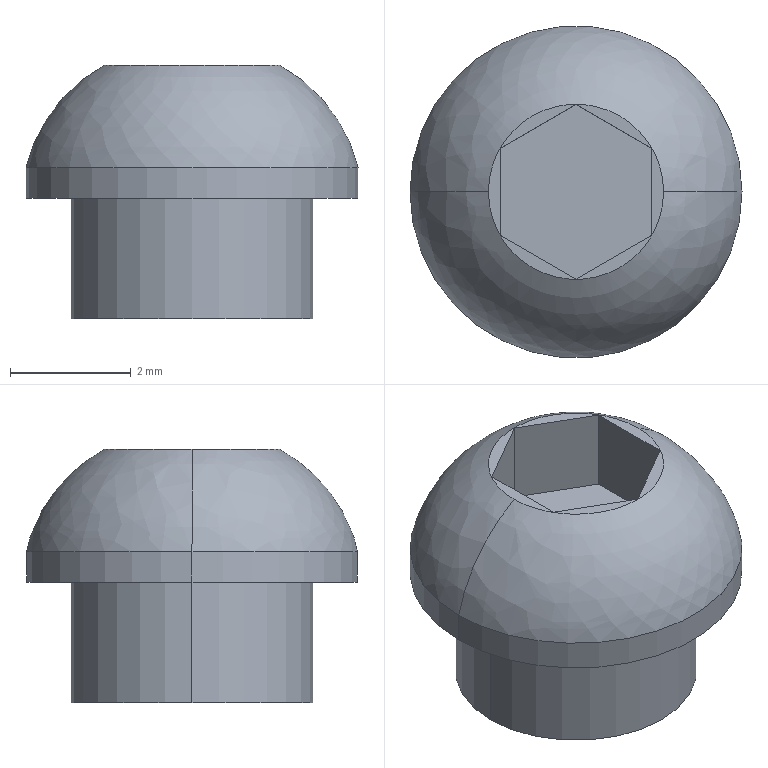Part | STEP file | 1 solid | 16 faces | box 5.5 x 5.5 x 4.2 mm | volume 58.227 mm3 | plane 10 | cylinder 4 | spline 2 | commonest cylinder face diameters 4 x2 5.5 x2
STEP:
#1=CARTESIAN_POINT('',(0.,0.,0.));
#2=DIRECTION('',(0.,0.,1.));
#3=DIRECTION('',(1.,0.,0.));
#4=AXIS2_PLACEMENT_3D('',#1,#2,#3);
#5=CARTESIAN_POINT('',(2.735,0.,5.794));
#6=VERTEX_POINT('',#5);
#7=CARTESIAN_POINT('',(-0.1645,0.,5.794));
#8=VERTEX_POINT('',#7);
#9=CARTESIAN_POINT('',(1.285,0.,5.794));
#10=DIRECTION('',(0.,0.,-1.));
#11=DIRECTION('',(1.,0.,0.));
#12=AXIS2_PLACEMENT_3D('',#9,#10,#11);
#13=CIRCLE('',#12,1.45);
#14=CARTESIAN_POINT('',(-0.1645,0.,5.794));
#15=CARTESIAN_POINT('',(-0.1645,-2.9,5.794));
#16=CARTESIAN_POINT('',(2.735,-2.9,5.794));
#17=CARTESIAN_POINT('',(2.735,0.,5.794));
#18=CARTESIAN_POINT('',(-0.8301,0.,5.432));
#19=CARTESIAN_POINT('',(-0.8301,-4.231,5.432));
#20=CARTESIAN_POINT('',(3.401,-4.231,5.432));
#21=CARTESIAN_POINT('',(3.401,0.,5.432));
#22=CARTESIAN_POINT('',(-1.29,0.,4.831));
#23=CARTESIAN_POINT('',(-1.29,-5.151,4.831));
#24=CARTESIAN_POINT('',(3.861,-5.151,4.831));
#25=CARTESIAN_POINT('',(3.861,0.,4.831));
#26=CARTESIAN_POINT('',(-1.465,0.,4.094));
#27=CARTESIAN_POINT('',(-1.465,-5.5,4.094));
#28=CARTESIAN_POINT('',(4.035,-5.5,4.094));
#29=CARTESIAN_POINT('',(4.035,0.,4.094));
#30=(BOUNDED_SURFACE()B_SPLINE_SURFACE(3,3,((#14,#15,#16,#17),(#18,#19,#20,#21),(#22,#23,#24,#25),(#26,#27,#28,#29)),.UNSPECIFIED.,.F.,.F.,.F.)B_SPLINE_SURFACE_WITH_KNOTS((4,4),(4,4),(0.,1.),(0.,1.),.PIECEWISE_BEZIER_KNOTS.)GEOMETRIC_REPRESENTATION_ITEM()RATIONAL_B_SPLINE_SURFACE(((1.,0.3333,0.3333,1.),(0.9419,0.314,0.314,0.9419),(0.9419,0.314,0.314,0.9419),(1.,0.3333,0.3333,1.)))REPRESENTATION_ITEM('')SURFACE());
#31=CARTESIAN_POINT('',(0.,1.));
#32=CARTESIAN_POINT('',(0.,0.9763));
#33=CARTESIAN_POINT('',(0.,0.9319));
#34=CARTESIAN_POINT('',(0.,0.8733));
#35=CARTESIAN_POINT('',(0.,0.8206));
#36=CARTESIAN_POINT('',(0.,0.7724));
#37=CARTESIAN_POINT('',(0.,0.7279));
#38=CARTESIAN_POINT('',(0.,0.6861));
#39=CARTESIAN_POINT('',(0.,0.6465));
#40=CARTESIAN_POINT('',(0.,0.6086));
#41=CARTESIAN_POINT('',(0.,0.5718));
#42=CARTESIAN_POINT('',(0.,0.5357));
#43=CARTESIAN_POINT('',(0.,0.5));
#44=CARTESIAN_POINT('',(0.,0.4643));
#45=CARTESIAN_POINT('',(0.,0.4282));
#46=CARTESIAN_POINT('',(0.,0.3914));
#47=CARTESIAN_POINT('',(0.,0.3535));
#48=CARTESIAN_POINT('',(0.,0.3139));
#49=CARTESIAN_POINT('',(0.,0.2721));
#50=CARTESIAN_POINT('',(0.,0.2276));
#51=CARTESIAN_POINT('',(0.,0.1794));
#52=CARTESIAN_POINT('',(0.,0.1267));
#53=CARTESIAN_POINT('',(0.,0.06805));
#54=CARTESIAN_POINT('',(0.,0.02375));
#55=CARTESIAN_POINT('',(0.,0.));
#56=B_SPLINE_CURVE_WITH_KNOTS('',3,(#31,#32,#33,#34,#35,#36,#37,#38,#39,#40,#41,#42,#43,#44,#45,#46,#47,#48,#49,#50,#51,#52,#53,#54,#55),.UNSPECIFIED.,.F.,.F.,(4,1,1,1,1,1,1,1,1,1,1,1,1,1,1,1,1,1,1,1,1,1,4),(0.,0.1428,0.2856,0.4284,0.5712,0.714,0.8568,0.9996,1.142,1.285,1.428,1.571,1.714,1.856,1.999,2.142,2.285,2.428,2.57,2.713,2.856,2.999,3.142),.QUASI_UNIFORM_KNOTS.);
#57=(GEOMETRIC_REPRESENTATION_CONTEXT(2)PARAMETRIC_REPRESENTATION_CONTEXT()REPRESENTATION_CONTEXT('',''));
#58=DEFINITIONAL_REPRESENTATION('',(#56),#57);
#59=PCURVE('',#30,#58);
#60=CARTESIAN_POINT('',(1.285,0.,5.794));
#61=DIRECTION('',(0.,0.,1.));
#62=DIRECTION('',(1.,0.,0.));
#63=AXIS2_PLACEMENT_3D('',#60,#61,#62);
#64=PLANE('',#63);
#65=CARTESIAN_POINT('',(1.45,0.));
#66=CARTESIAN_POINT('',(1.45,-2.511));
#67=CARTESIAN_POINT('',(-0.725,-1.256));
#68=CARTESIAN_POINT('',(-2.9,0.));
#69=CARTESIAN_POINT('',(-0.725,1.256));
#70=CARTESIAN_POINT('',(1.45,2.511));
#71=CARTESIAN_POINT('',(1.45,0.));
#72=(BOUNDED_CURVE()B_SPLINE_CURVE(2,(#65,#66,#67,#68,#69,#70,#71),.UNSPECIFIED.,.T.,.F.)B_SPLINE_CURVE_WITH_KNOTS((1,2,2,2,2,1),(-2.094,0.,2.094,4.189,6.283,8.378),.UNSPECIFIED.)CURVE()GEOMETRIC_REPRESENTATION_ITEM()RATIONAL_B_SPLINE_CURVE((1.,0.5,1.,0.5,1.,0.5,1.))REPRESENTATION_ITEM(''));
#73=(GEOMETRIC_REPRESENTATION_CONTEXT(2)PARAMETRIC_REPRESENTATION_CONTEXT()REPRESENTATION_CONTEXT('',''));
#74=DEFINITIONAL_REPRESENTATION('',(#72),#73);
#75=PCURVE('',#64,#74);
#76=SURFACE_CURVE('',#13,(#59,#75),.PCURVE_S1.);
#77=EDGE_CURVE('',#6,#8,#76,.T.);
#78=ORIENTED_EDGE('',*,*,#77,.T.);
#79=CARTESIAN_POINT('',(-1.465,0.,4.094));
#80=VERTEX_POINT('',#79);
#81=CARTESIAN_POINT('',(1.086,0.,3.49));
#82=DIRECTION('',(0.,-1.,0.));
#83=DIRECTION('',(-1.,0.,0.));
#84=AXIS2_PLACEMENT_3D('',#81,#82,#83);
#85=CIRCLE('',#84,2.621);
#86=CARTESIAN_POINT('',(0.,0.));
#87=CARTESIAN_POINT('',(1.,0.));
#88=B_SPLINE_CURVE_WITH_KNOTS('',1,(#86,#87),.UNSPECIFIED.,.F.,.F.,(2,2),(5.21,6.051),.PIECEWISE_BEZIER_KNOTS.);
#89=(GEOMETRIC_REPRESENTATION_CONTEXT(2)PARAMETRIC_REPRESENTATION_CONTEXT()REPRESENTATION_CONTEXT('',''));
#90=DEFINITIONAL_REPRESENTATION('',(#88),#89);
#91=PCURVE('',#30,#90);
#92=CARTESIAN_POINT('',(2.735,0.,5.794));
#93=CARTESIAN_POINT('',(2.735,2.9,5.794));
#94=CARTESIAN_POINT('',(-0.1645,2.9,5.794));
#95=CARTESIAN_POINT('',(-0.1645,0.,5.794));
#96=CARTESIAN_POINT('',(3.401,0.,5.432));
#97=CARTESIAN_POINT('',(3.401,4.231,5.432));
#98=CARTESIAN_POINT('',(-0.8301,4.231,5.432));
#99=CARTESIAN_POINT('',(-0.8301,0.,5.432));
#100=CARTESIAN_POINT('',(3.861,0.,4.831));
#101=CARTESIAN_POINT('',(3.861,5.151,4.831));
#102=CARTESIAN_POINT('',(-1.29,5.151,4.831));
#103=CARTESIAN_POINT('',(-1.29,0.,4.831));
#104=CARTESIAN_POINT('',(4.035,0.,4.094));
#105=CARTESIAN_POINT('',(4.035,5.5,4.094));
#106=CARTESIAN_POINT('',(-1.465,5.5,4.094));
#107=CARTESIAN_POINT('',(-1.465,0.,4.094));
#108=(BOUNDED_SURFACE()B_SPLINE_SURFACE(3,3,((#92,#93,#94,#95),(#96,#97,#98,#99),(#100,#101,#102,#103),(#104,#105,#106,#107)),.UNSPECIFIED.,.F.,.F.,.F.)B_SPLINE_SURFACE_WITH_KNOTS((4,4),(4,4),(0.,1.),(0.,1.),.PIECEWISE_BEZIER_KNOTS.)GEOMETRIC_REPRESENTATION_ITEM()RATIONAL_B_SPLINE_SURFACE(((1.,0.3333,0.3333,1.),(0.9419,0.314,0.314,0.9419),(0.9419,0.314,0.314,0.9419),(1.,0.3333,0.3333,1.)))REPRESENTATION_ITEM('')SURFACE());
#109=CARTESIAN_POINT('',(0.,1.));
#110=CARTESIAN_POINT('',(1.,1.));
#111=B_SPLINE_CURVE_WITH_KNOTS('',1,(#109,#110),.UNSPECIFIED.,.F.,.F.,(2,2),(5.21,6.051),.PIECEWISE_BEZIER_KNOTS.);
#112=(GEOMETRIC_REPRESENTATION_CONTEXT(2)PARAMETRIC_REPRESENTATION_CONTEXT()REPRESENTATION_CONTEXT('',''));
#113=DEFINITIONAL_REPRESENTATION('',(#111),#112);
#114=PCURVE('',#108,#113);
#115=SURFACE_CURVE('',#85,(#91,#114),.PCURVE_S1.);
#116=EDGE_CURVE('',#8,#80,#115,.T.);
#117=ORIENTED_EDGE('',*,*,#116,.T.);
#118=CARTESIAN_POINT('',(4.035,0.,4.094));
#119=VERTEX_POINT('',#118);
#120=CARTESIAN_POINT('',(1.285,0.,4.094));
#121=DIRECTION('',(0.,0.,1.));
#122=DIRECTION('',(1.,0.,0.));
#123=AXIS2_PLACEMENT_3D('',#120,#121,#122);
#124=CIRCLE('',#123,2.75);
#125=CARTESIAN_POINT('',(1.,0.));
#126=CARTESIAN_POINT('',(1.,0.02375));
#127=CARTESIAN_POINT('',(1.,0.06805));
#128=CARTESIAN_POINT('',(1.,0.1267));
#129=CARTESIAN_POINT('',(1.,0.1794));
#130=CARTESIAN_POINT('',(1.,0.2276));
#131=CARTESIAN_POINT('',(1.,0.2721));
#132=CARTESIAN_POINT('',(1.,0.3139));
#133=CARTESIAN_POINT('',(1.,0.3535));
#134=CARTESIAN_POINT('',(1.,0.3914));
#135=CARTESIAN_POINT('',(1.,0.4282));
#136=CARTESIAN_POINT('',(1.,0.4643));
#137=CARTESIAN_POINT('',(1.,0.5));
#138=CARTESIAN_POINT('',(1.,0.5357));
#139=CARTESIAN_POINT('',(1.,0.5718));
#140=CARTESIAN_POINT('',(1.,0.6086));
#141=CARTESIAN_POINT('',(1.,0.6465));
#142=CARTESIAN_POINT('',(1.,0.6861));
#143=CARTESIAN_POINT('',(1.,0.7279));
#144=CARTESIAN_POINT('',(1.,0.7724));
#145=CARTESIAN_POINT('',(1.,0.8206));
#146=CARTESIAN_POINT('',(1.,0.8733));
#147=CARTESIAN_POINT('',(1.,0.9319));
#148=CARTESIAN_POINT('',(1.,0.9763));
#149=CARTESIAN_POINT('',(1.,1.));
#150=B_SPLINE_CURVE_WITH_KNOTS('',3,(#125,#126,#127,#128,#129,#130,#131,#132,#133,#134,#135,#136,#137,#138,#139,#140,#141,#142,#143,#144,#145,#146,#147,#148,#149),.UNSPECIFIED.,.F.,.F.,(4,1,1,1,1,1,1,1,1,1,1,1,1,1,1,1,1,1,1,1,1,1,4),(3.142,3.284,3.427,3.57,3.713,3.856,3.998,4.141,4.284,4.427,4.57,4.712,4.855,4.998,5.141,5.284,5.426,5.569,5.712,5.855,5.998,6.14,6.283),.QUASI_UNIFORM_KNOTS.);
#151=(GEOMETRIC_REPRESENTATION_CONTEXT(2)PARAMETRIC_REPRESENTATION_CONTEXT()REPRESENTATION_CONTEXT('',''));
#152=DEFINITIONAL_REPRESENTATION('',(#150),#151);
#153=PCURVE('',#30,#152);
#154=CARTESIAN_POINT('',(1.285,0.,3.844));
#155=DIRECTION('',(0.,0.,-1.));
#156=DIRECTION('',(-1.,0.,0.));
#157=AXIS2_PLACEMENT_3D('',#154,#155,#156);
#158=CYLINDRICAL_SURFACE('',#157,2.75);
#159=CARTESIAN_POINT('',(9.425,-0.25));
#160=DIRECTION('',(-1.,0.));
#161=VECTOR('',#160,1.);
#162=LINE('',#159,#161);
#163=(GEOMETRIC_REPRESENTATION_CONTEXT(2)PARAMETRIC_REPRESENTATION_CONTEXT()REPRESENTATION_CONTEXT('',''));
#164=DEFINITIONAL_REPRESENTATION('',(#162),#163);
#165=PCURVE('',#158,#164);
#166=SURFACE_CURVE('',#124,(#153,#165),.PCURVE_S1.);
#167=EDGE_CURVE('',#80,#119,#166,.T.);
#168=ORIENTED_EDGE('',*,*,#167,.T.);
#169=CARTESIAN_POINT('',(1.485,0.,3.49));
#170=DIRECTION('',(0.,1.,0.));
#171=DIRECTION('',(1.,0.,0.));
#172=AXIS2_PLACEMENT_3D('',#169,#170,#171);
#173=CIRCLE('',#172,2.621);
#174=CARTESIAN_POINT('',(0.,1.));
#175=CARTESIAN_POINT('',(1.,1.));
#176=B_SPLINE_CURVE_WITH_KNOTS('',1,(#174,#175),.UNSPECIFIED.,.F.,.F.,(2,2),(5.21,6.051),.PIECEWISE_BEZIER_KNOTS.);
#177=(GEOMETRIC_REPRESENTATION_CONTEXT(2)PARAMETRIC_REPRESENTATION_CONTEXT()REPRESENTATION_CONTEXT('',''));
#178=DEFINITIONAL_REPRESENTATION('',(#176),#177);
#179=PCURVE('',#30,#178);
#180=CARTESIAN_POINT('',(0.,0.));
#181=CARTESIAN_POINT('',(1.,0.));
#182=B_SPLINE_CURVE_WITH_KNOTS('',1,(#180,#181),.UNSPECIFIED.,.F.,.F.,(2,2),(5.21,6.051),.PIECEWISE_BEZIER_KNOTS.);
#183=(GEOMETRIC_REPRESENTATION_CONTEXT(2)PARAMETRIC_REPRESENTATION_CONTEXT()REPRESENTATION_CONTEXT('',''));
#184=DEFINITIONAL_REPRESENTATION('',(#182),#183);
#185=PCURVE('',#108,#184);
#186=SURFACE_CURVE('',#173,(#179,#185),.PCURVE_S1.);
#187=EDGE_CURVE('',#6,#119,#186,.T.);
#188=ORIENTED_EDGE('',*,*,#187,.F.);
#189=EDGE_LOOP('',(#78,#117,#168,#188));
#190=FACE_BOUND('',#189,.T.);
#191=ADVANCED_FACE('',(#190),#30,.T.);
#192=CARTESIAN_POINT('',(1.285,0.,4.094));
#193=DIRECTION('',(0.,0.,1.));
#194=DIRECTION('',(1.,0.,0.));
#195=AXIS2_PLACEMENT_3D('',#192,#193,#194);
#196=CIRCLE('',#195,2.75);
#197=CARTESIAN_POINT('',(1.285,0.,3.844));
#198=DIRECTION('',(0.,0.,-1.));
#199=DIRECTION('',(-1.,0.,0.));
#200=AXIS2_PLACEMENT_3D('',#197,#198,#199);
#201=CYLINDRICAL_SURFACE('',#200,2.75);
#202=CARTESIAN_POINT('',(3.142,-0.25));
#203=DIRECTION('',(-1.,0.));
#204=VECTOR('',#203,1.);
#205=LINE('',#202,#204);
#206=(GEOMETRIC_REPRESENTATION_CONTEXT(2)PARAMETRIC_REPRESENTATION_CONTEXT()REPRESENTATION_CONTEXT('',''));
#207=DEFINITIONAL_REPRESENTATION('',(#205),#206);
#208=PCURVE('',#201,#207);
#209=CARTESIAN_POINT('',(1.,0.));
#210=CARTESIAN_POINT('',(1.,0.02375));
#211=CARTESIAN_POINT('',(1.,0.06805));
#212=CARTESIAN_POINT('',(1.,0.1267));
#213=CARTESIAN_POINT('',(1.,0.1794));
#214=CARTESIAN_POINT('',(1.,0.2276));
#215=CARTESIAN_POINT('',(1.,0.2721));
#216=CARTESIAN_POINT('',(1.,0.3139));
#217=CARTESIAN_POINT('',(1.,0.3535));
#218=CARTESIAN_POINT('',(1.,0.3914));
#219=CARTESIAN_POINT('',(1.,0.4282));
#220=CARTESIAN_POINT('',(1.,0.4643));
#221=CARTESIAN_POINT('',(1.,0.5));
#222=CARTESIAN_POINT('',(1.,0.5357));
#223=CARTESIAN_POINT('',(1.,0.5718));
#224=CARTESIAN_POINT('',(1.,0.6086));
#225=CARTESIAN_POINT('',(1.,0.6465));
#226=CARTESIAN_POINT('',(1.,0.6861));
#227=CARTESIAN_POINT('',(1.,0.7279));
#228=CARTESIAN_POINT('',(1.,0.7724));
#229=CARTESIAN_POINT('',(1.,0.8206));
#230=CARTESIAN_POINT('',(1.,0.8733));
#231=CARTESIAN_POINT('',(1.,0.9319));
#232=CARTESIAN_POINT('',(1.,0.9763));
#233=CARTESIAN_POINT('',(1.,1.));
#234=B_SPLINE_CURVE_WITH_KNOTS('',3,(#209,#210,#211,#212,#213,#214,#215,#216,#217,#218,#219,#220,#221,#222,#223,#224,#225,#226,#227,#228,#229,#230,#231,#232,#233),.UNSPECIFIED.,.F.,.F.,(4,1,1,1,1,1,1,1,1,1,1,1,1,1,1,1,1,1,1,1,1,1,4),(0.,0.1428,0.2856,0.4284,0.5712,0.714,0.8568,0.9996,1.142,1.285,1.428,1.571,1.714,1.856,1.999,2.142,2.285,2.428,2.57,2.713,2.856,2.999,3.142),.QUASI_UNIFORM_KNOTS.);
#235=(GEOMETRIC_REPRESENTATION_CONTEXT(2)PARAMETRIC_REPRESENTATION_CONTEXT()REPRESENTATION_CONTEXT('',''));
#236=DEFINITIONAL_REPRESENTATION('',(#234),#235);
#237=PCURVE('',#108,#236);
#238=SURFACE_CURVE('',#196,(#208,#237),.PCURVE_S1.);
#239=EDGE_CURVE('',#119,#80,#238,.T.);
#240=ORIENTED_EDGE('',*,*,#239,.F.);
#241=CARTESIAN_POINT('',(4.035,0.,3.594));
#242=VERTEX_POINT('',#241);
#243=CARTESIAN_POINT('',(4.035,0.,3.844));
#244=DIRECTION('',(0.,0.,-1.));
#245=VECTOR('',#244,1.);
#246=LINE('',#243,#245);
#247=CARTESIAN_POINT('',(3.142,0.));
#248=DIRECTION('',(0.,1.));
#249=VECTOR('',#248,1.);
#250=LINE('',#247,#249);
#251=(GEOMETRIC_REPRESENTATION_CONTEXT(2)PARAMETRIC_REPRESENTATION_CONTEXT()REPRESENTATION_CONTEXT('',''));
#252=DEFINITIONAL_REPRESENTATION('',(#250),#251);
#253=PCURVE('',#201,#252);
#254=CARTESIAN_POINT('',(3.142,0.));
#255=DIRECTION('',(0.,1.));
#256=VECTOR('',#255,1.);
#257=LINE('',#254,#256);
#258=(GEOMETRIC_REPRESENTATION_CONTEXT(2)PARAMETRIC_REPRESENTATION_CONTEXT()REPRESENTATION_CONTEXT('',''));
#259=DEFINITIONAL_REPRESENTATION('',(#257),#258);
#260=PCURVE('',#158,#259);
#261=SURFACE_CURVE('',#246,(#253,#260),.PCURVE_S1.);
#262=EDGE_CURVE('',#119,#242,#261,.T.);
#263=ORIENTED_EDGE('',*,*,#262,.T.);
#264=CARTESIAN_POINT('',(-1.465,0.,3.594));
#265=VERTEX_POINT('',#264);
#266=CARTESIAN_POINT('',(1.285,0.,3.594));
#267=DIRECTION('',(0.,0.,1.));
#268=DIRECTION('',(-1.,0.,0.));
#269=AXIS2_PLACEMENT_3D('',#266,#267,#268);
#270=CIRCLE('',#269,2.75);
#271=CARTESIAN_POINT('',(6.283,0.25));
#272=DIRECTION('',(-1.,0.));
#273=VECTOR('',#272,1.);
#274=LINE('',#271,#273);
#275=(GEOMETRIC_REPRESENTATION_CONTEXT(2)PARAMETRIC_REPRESENTATION_CONTEXT()REPRESENTATION_CONTEXT('',''));
#276=DEFINITIONAL_REPRESENTATION('',(#274),#275);
#277=PCURVE('',#201,#276);
#278=CARTESIAN_POINT('',(4.035,0.,3.594));
#279=DIRECTION('',(0.,0.,-1.));
#280=DIRECTION('',(-1.,0.,0.));
#281=AXIS2_PLACEMENT_3D('',#278,#279,#280);
#282=PLANE('',#281);
#283=CARTESIAN_POINT('',(5.5,0.));
#284=CARTESIAN_POINT('',(5.5,-4.763));
#285=CARTESIAN_POINT('',(1.375,-2.382));
#286=CARTESIAN_POINT('',(-2.75,0.));
#287=CARTESIAN_POINT('',(1.375,2.382));
#288=CARTESIAN_POINT('',(5.5,4.763));
#289=CARTESIAN_POINT('',(5.5,0.));
#290=(BOUNDED_CURVE()B_SPLINE_CURVE(2,(#283,#284,#285,#286,#287,#288,#289),.UNSPECIFIED.,.T.,.F.)B_SPLINE_CURVE_WITH_KNOTS((1,2,2,2,2,1),(-2.094,0.,2.094,4.189,6.283,8.378),.UNSPECIFIED.)CURVE()GEOMETRIC_REPRESENTATION_ITEM()RATIONAL_B_SPLINE_CURVE((1.,0.5,1.,0.5,1.,0.5,1.))REPRESENTATION_ITEM(''));
#291=(GEOMETRIC_REPRESENTATION_CONTEXT(2)PARAMETRIC_REPRESENTATION_CONTEXT()REPRESENTATION_CONTEXT('',''));
#292=DEFINITIONAL_REPRESENTATION('',(#290),#291);
#293=PCURVE('',#282,#292);
#294=SURFACE_CURVE('',#270,(#277,#293),.PCURVE_S1.);
#295=EDGE_CURVE('',#242,#265,#294,.T.);
#296=ORIENTED_EDGE('',*,*,#295,.T.);
#297=CARTESIAN_POINT('',(-1.465,0.,3.844));
#298=DIRECTION('',(0.,0.,-1.));
#299=VECTOR('',#298,1.);
#300=LINE('',#297,#299);
#301=CARTESIAN_POINT('',(0.,0.));
#302=DIRECTION('',(0.,1.));
#303=VECTOR('',#302,1.);
#304=LINE('',#301,#303);
#305=(GEOMETRIC_REPRESENTATION_CONTEXT(2)PARAMETRIC_REPRESENTATION_CONTEXT()REPRESENTATION_CONTEXT('',''));
#306=DEFINITIONAL_REPRESENTATION('',(#304),#305);
#307=PCURVE('',#201,#306);
#308=CARTESIAN_POINT('',(6.283,0.));
#309=DIRECTION('',(0.,1.));
#310=VECTOR('',#309,1.);
#311=LINE('',#308,#310);
#312=(GEOMETRIC_REPRESENTATION_CONTEXT(2)PARAMETRIC_REPRESENTATION_CONTEXT()REPRESENTATION_CONTEXT('',''));
#313=DEFINITIONAL_REPRESENTATION('',(#311),#312);
#314=PCURVE('',#158,#313);
#315=SURFACE_CURVE('',#300,(#307,#314),.PCURVE_S1.);
#316=EDGE_CURVE('',#80,#265,#315,.T.);
#317=ORIENTED_EDGE('',*,*,#316,.F.);
#318=EDGE_LOOP('',(#240,#263,#296,#317));
#319=FACE_BOUND('',#318,.T.);
#320=ADVANCED_FACE('',(#319),#201,.T.);
#321=CARTESIAN_POINT('',(3.285,0.,3.594));
#322=VERTEX_POINT('',#321);
#323=CARTESIAN_POINT('',(-0.7145,0.,3.594));
#324=VERTEX_POINT('',#323);
#325=CARTESIAN_POINT('',(1.285,0.,3.594));
#326=DIRECTION('',(0.,0.,1.));
#327=DIRECTION('',(-1.,0.,0.));
#328=AXIS2_PLACEMENT_3D('',#325,#326,#327);
#329=CIRCLE('',#328,2.);
#330=CARTESIAN_POINT('',(1.285,0.,2.594));
#331=DIRECTION('',(0.,0.,-1.));
#332=DIRECTION('',(-1.,0.,0.));
#333=AXIS2_PLACEMENT_3D('',#330,#331,#332);
#334=CYLINDRICAL_SURFACE('',#333,2.);
#335=CARTESIAN_POINT('',(6.283,-1.));
#336=DIRECTION('',(-1.,0.));
#337=VECTOR('',#336,1.);
#338=LINE('',#335,#337);
#339=(GEOMETRIC_REPRESENTATION_CONTEXT(2)PARAMETRIC_REPRESENTATION_CONTEXT()REPRESENTATION_CONTEXT('',''));
#340=DEFINITIONAL_REPRESENTATION('',(#338),#339);
#341=PCURVE('',#334,#340);
#342=CARTESIAN_POINT('',(4.75,0.));
#343=CARTESIAN_POINT('',(4.75,-3.464));
#344=CARTESIAN_POINT('',(1.75,-1.732));
#345=CARTESIAN_POINT('',(-1.25,0.));
#346=CARTESIAN_POINT('',(1.75,1.732));
#347=CARTESIAN_POINT('',(4.75,3.464));
#348=CARTESIAN_POINT('',(4.75,0.));
#349=(BOUNDED_CURVE()B_SPLINE_CURVE(2,(#342,#343,#344,#345,#346,#347,#348),.UNSPECIFIED.,.T.,.F.)B_SPLINE_CURVE_WITH_KNOTS((1,2,2,2,2,1),(-2.094,0.,2.094,4.189,6.283,8.378),.UNSPECIFIED.)CURVE()GEOMETRIC_REPRESENTATION_ITEM()RATIONAL_B_SPLINE_CURVE((1.,0.5,1.,0.5,1.,0.5,1.))REPRESENTATION_ITEM(''));
#350=(GEOMETRIC_REPRESENTATION_CONTEXT(2)PARAMETRIC_REPRESENTATION_CONTEXT()REPRESENTATION_CONTEXT('',''));
#351=DEFINITIONAL_REPRESENTATION('',(#349),#350);
#352=PCURVE('',#282,#351);
#353=SURFACE_CURVE('',#329,(#341,#352),.PCURVE_S1.);
#354=EDGE_CURVE('',#322,#324,#353,.T.);
#355=ORIENTED_EDGE('',*,*,#354,.F.);
#356=CARTESIAN_POINT('',(3.285,0.,1.594));
#357=VERTEX_POINT('',#356);
#358=CARTESIAN_POINT('',(3.285,0.,2.594));
#359=DIRECTION('',(0.,0.,-1.));
#360=VECTOR('',#359,1.);
#361=LINE('',#358,#360);
#362=CARTESIAN_POINT('',(3.142,0.));
#363=DIRECTION('',(0.,1.));
#364=VECTOR('',#363,1.);
#365=LINE('',#362,#364);
#366=(GEOMETRIC_REPRESENTATION_CONTEXT(2)PARAMETRIC_REPRESENTATION_CONTEXT()REPRESENTATION_CONTEXT('',''));
#367=DEFINITIONAL_REPRESENTATION('',(#365),#366);
#368=PCURVE('',#334,#367);
#369=CARTESIAN_POINT('',(1.285,0.,2.594));
#370=DIRECTION('',(0.,0.,-1.));
#371=DIRECTION('',(-1.,0.,0.));
#372=AXIS2_PLACEMENT_3D('',#369,#370,#371);
#373=CYLINDRICAL_SURFACE('',#372,2.);
#374=CARTESIAN_POINT('',(3.142,0.));
#375=DIRECTION('',(0.,1.));
#376=VECTOR('',#375,1.);
#377=LINE('',#374,#376);
#378=(GEOMETRIC_REPRESENTATION_CONTEXT(2)PARAMETRIC_REPRESENTATION_CONTEXT()REPRESENTATION_CONTEXT('',''));
#379=DEFINITIONAL_REPRESENTATION('',(#377),#378);
#380=PCURVE('',#373,#379);
#381=SURFACE_CURVE('',#361,(#368,#380),.PCURVE_S1.);
#382=EDGE_CURVE('',#322,#357,#381,.T.);
#383=ORIENTED_EDGE('',*,*,#382,.T.);
#384=CARTESIAN_POINT('',(-0.7145,0.,1.594));
#385=VERTEX_POINT('',#384);
#386=CARTESIAN_POINT('',(1.285,0.,1.594));
#387=DIRECTION('',(0.,0.,1.));
#388=DIRECTION('',(-1.,0.,0.));
#389=AXIS2_PLACEMENT_3D('',#386,#387,#388);
#390=CIRCLE('',#389,2.);
#391=CARTESIAN_POINT('',(6.283,1.));
#392=DIRECTION('',(-1.,0.));
#393=VECTOR('',#392,1.);
#394=LINE('',#391,#393);
#395=(GEOMETRIC_REPRESENTATION_CONTEXT(2)PARAMETRIC_REPRESENTATION_CONTEXT()REPRESENTATION_CONTEXT('',''));
#396=DEFINITIONAL_REPRESENTATION('',(#394),#395);
#397=PCURVE('',#334,#396);
#398=CARTESIAN_POINT('',(3.285,0.,1.594));
#399=DIRECTION('',(0.,0.,-1.));
#400=DIRECTION('',(-1.,0.,0.));
#401=AXIS2_PLACEMENT_3D('',#398,#399,#400);
#402=PLANE('',#401);
#403=CARTESIAN_POINT('',(4.,0.));
#404=CARTESIAN_POINT('',(4.,-3.464));
#405=CARTESIAN_POINT('',(1.,-1.732));
#406=CARTESIAN_POINT('',(-2.,0.));
#407=CARTESIAN_POINT('',(1.,1.732));
#408=CARTESIAN_POINT('',(4.,3.464));
#409=CARTESIAN_POINT('',(4.,0.));
#410=(BOUNDED_CURVE()B_SPLINE_CURVE(2,(#403,#404,#405,#406,#407,#408,#409),.UNSPECIFIED.,.T.,.F.)B_SPLINE_CURVE_WITH_KNOTS((1,2,2,2,2,1),(-2.094,0.,2.094,4.189,6.283,8.378),.UNSPECIFIED.)CURVE()GEOMETRIC_REPRESENTATION_ITEM()RATIONAL_B_SPLINE_CURVE((1.,0.5,1.,0.5,1.,0.5,1.))REPRESENTATION_ITEM(''));
#411=(GEOMETRIC_REPRESENTATION_CONTEXT(2)PARAMETRIC_REPRESENTATION_CONTEXT()REPRESENTATION_CONTEXT('',''));
#412=DEFINITIONAL_REPRESENTATION('',(#410),#411);
#413=PCURVE('',#402,#412);
#414=SURFACE_CURVE('',#390,(#397,#413),.PCURVE_S1.);
#415=EDGE_CURVE('',#357,#385,#414,.T.);
#416=ORIENTED_EDGE('',*,*,#415,.T.);
#417=CARTESIAN_POINT('',(-0.7145,0.,2.594));
#418=DIRECTION('',(0.,0.,-1.));
#419=VECTOR('',#418,1.);
#420=LINE('',#417,#419);
#421=CARTESIAN_POINT('',(0.,0.));
#422=DIRECTION('',(0.,1.));
#423=VECTOR('',#422,1.);
#424=LINE('',#421,#423);
#425=(GEOMETRIC_REPRESENTATION_CONTEXT(2)PARAMETRIC_REPRESENTATION_CONTEXT()REPRESENTATION_CONTEXT('',''));
#426=DEFINITIONAL_REPRESENTATION('',(#424),#425);
#427=PCURVE('',#334,#426);
#428=CARTESIAN_POINT('',(6.283,0.));
#429=DIRECTION('',(0.,1.));
#430=VECTOR('',#429,1.);
#431=LINE('',#428,#430);
#432=(GEOMETRIC_REPRESENTATION_CONTEXT(2)PARAMETRIC_REPRESENTATION_CONTEXT()REPRESENTATION_CONTEXT('',''));
#433=DEFINITIONAL_REPRESENTATION('',(#431),#432);
#434=PCURVE('',#373,#433);
#435=SURFACE_CURVE('',#420,(#427,#434),.PCURVE_S1.);
#436=EDGE_CURVE('',#324,#385,#435,.T.);
#437=ORIENTED_EDGE('',*,*,#436,.F.);
#438=EDGE_LOOP('',(#355,#383,#416,#437));
#439=FACE_BOUND('',#438,.T.);
#440=ADVANCED_FACE('',(#439),#334,.T.);
#441=ORIENTED_EDGE('',*,*,#116,.F.);
#442=CARTESIAN_POINT('',(1.285,0.,5.794));
#443=DIRECTION('',(0.,0.,-1.));
#444=DIRECTION('',(1.,0.,0.));
#445=AXIS2_PLACEMENT_3D('',#442,#443,#444);
#446=CIRCLE('',#445,1.45);
#447=CARTESIAN_POINT('',(0.,1.));
#448=CARTESIAN_POINT('',(0.,0.9763));
#449=CARTESIAN_POINT('',(0.,0.9319));
#450=CARTESIAN_POINT('',(0.,0.8733));
#451=CARTESIAN_POINT('',(0.,0.8206));
#452=CARTESIAN_POINT('',(0.,0.7724));
#453=CARTESIAN_POINT('',(0.,0.7279));
#454=CARTESIAN_POINT('',(0.,0.6861));
#455=CARTESIAN_POINT('',(0.,0.6465));
#456=CARTESIAN_POINT('',(0.,0.6086));
#457=CARTESIAN_POINT('',(0.,0.5718));
#458=CARTESIAN_POINT('',(0.,0.5357));
#459=CARTESIAN_POINT('',(0.,0.5));
#460=CARTESIAN_POINT('',(0.,0.4643));
#461=CARTESIAN_POINT('',(0.,0.4282));
#462=CARTESIAN_POINT('',(0.,0.3914));
#463=CARTESIAN_POINT('',(0.,0.3535));
#464=CARTESIAN_POINT('',(0.,0.3139));
#465=CARTESIAN_POINT('',(0.,0.2721));
#466=CARTESIAN_POINT('',(0.,0.2276));
#467=CARTESIAN_POINT('',(0.,0.1794));
#468=CARTESIAN_POINT('',(0.,0.1267));
#469=CARTESIAN_POINT('',(0.,0.06805));
#470=CARTESIAN_POINT('',(0.,0.02375));
#471=CARTESIAN_POINT('',(0.,0.));
#472=B_SPLINE_CURVE_WITH_KNOTS('',3,(#447,#448,#449,#450,#451,#452,#453,#454,#455,#456,#457,#458,#459,#460,#461,#462,#463,#464,#465,#466,#467,#468,#469,#470,#471),.UNSPECIFIED.,.F.,.F.,(4,1,1,1,1,1,1,1,1,1,1,1,1,1,1,1,1,1,1,1,1,1,4),(3.142,3.284,3.427,3.57,3.713,3.856,3.998,4.141,4.284,4.427,4.57,4.712,4.855,4.998,5.141,5.284,5.426,5.569,5.712,5.855,5.998,6.14,6.283),.QUASI_UNIFORM_KNOTS.);
#473=(GEOMETRIC_REPRESENTATION_CONTEXT(2)PARAMETRIC_REPRESENTATION_CONTEXT()REPRESENTATION_CONTEXT('',''));
#474=DEFINITIONAL_REPRESENTATION('',(#472),#473);
#475=PCURVE('',#108,#474);
#476=CARTESIAN_POINT('',(1.45,0.));
#477=CARTESIAN_POINT('',(1.45,-2.511));
#478=CARTESIAN_POINT('',(-0.725,-1.256));
#479=CARTESIAN_POINT('',(-2.9,0.));
#480=CARTESIAN_POINT('',(-0.725,1.256));
#481=CARTESIAN_POINT('',(1.45,2.511));
#482=CARTESIAN_POINT('',(1.45,0.));
#483=(BOUNDED_CURVE()B_SPLINE_CURVE(2,(#476,#477,#478,#479,#480,#481,#482),.UNSPECIFIED.,.T.,.F.)B_SPLINE_CURVE_WITH_KNOTS((1,2,2,2,2,1),(-2.094,0.,2.094,4.189,6.283,8.378),.UNSPECIFIED.)CURVE()GEOMETRIC_REPRESENTATION_ITEM()RATIONAL_B_SPLINE_CURVE((1.,0.5,1.,0.5,1.,0.5,1.))REPRESENTATION_ITEM(''));
#484=(GEOMETRIC_REPRESENTATION_CONTEXT(2)PARAMETRIC_REPRESENTATION_CONTEXT()REPRESENTATION_CONTEXT('',''));
#485=DEFINITIONAL_REPRESENTATION('',(#483),#484);
#486=PCURVE('',#64,#485);
#487=SURFACE_CURVE('',#446,(#475,#486),.PCURVE_S1.);
#488=EDGE_CURVE('',#8,#6,#487,.T.);
#489=ORIENTED_EDGE('',*,*,#488,.T.);
#490=ORIENTED_EDGE('',*,*,#187,.T.);
#491=ORIENTED_EDGE('',*,*,#239,.T.);
#492=EDGE_LOOP('',(#441,#489,#490,#491));
#493=FACE_BOUND('',#492,.T.);
#494=ADVANCED_FACE('',(#493),#108,.T.);
#495=CARTESIAN_POINT('',(0.03548,0.7217,5.794));
#496=VERTEX_POINT('',#495);
#497=CARTESIAN_POINT('',(1.285,1.443,5.794));
#498=VERTEX_POINT('',#497);
#499=CARTESIAN_POINT('',(0.03548,0.7217,5.794));
#500=DIRECTION('',(0.866,0.5,0.));
#501=VECTOR('',#500,1.);
#502=LINE('',#499,#501);
#503=CARTESIAN_POINT('',(-1.25,0.7217));
#504=DIRECTION('',(0.866,0.5));
#505=VECTOR('',#504,1.);
#506=LINE('',#503,#505);
#507=(GEOMETRIC_REPRESENTATION_CONTEXT(2)PARAMETRIC_REPRESENTATION_CONTEXT()REPRESENTATION_CONTEXT('',''));
#508=DEFINITIONAL_REPRESENTATION('',(#506),#507);
#509=PCURVE('',#64,#508);
#510=CARTESIAN_POINT('',(0.03548,0.7217,5.794));
#511=DIRECTION('',(-0.5,0.866,0.));
#512=DIRECTION('',(-0.866,-0.5,0.));
#513=AXIS2_PLACEMENT_3D('',#510,#511,#512);
#514=PLANE('',#513);
#515=CARTESIAN_POINT('',(0.,0.));
#516=DIRECTION('',(-1.,0.));
#517=VECTOR('',#516,1.);
#518=LINE('',#515,#517);
#519=(GEOMETRIC_REPRESENTATION_CONTEXT(2)PARAMETRIC_REPRESENTATION_CONTEXT()REPRESENTATION_CONTEXT('',''));
#520=DEFINITIONAL_REPRESENTATION('',(#518),#519);
#521=PCURVE('',#514,#520);
#522=SURFACE_CURVE('',#502,(#509,#521),.PCURVE_S1.);
#523=EDGE_CURVE('',#496,#498,#522,.T.);
#524=ORIENTED_EDGE('',*,*,#523,.T.);
#525=CARTESIAN_POINT('',(2.535,0.7217,5.794));
#526=VERTEX_POINT('',#525);
#527=CARTESIAN_POINT('',(1.285,1.443,5.794));
#528=DIRECTION('',(0.866,-0.5,0.));
#529=VECTOR('',#528,1.);
#530=LINE('',#527,#529);
#531=CARTESIAN_POINT('',(0.,1.443));
#532=DIRECTION('',(0.866,-0.5));
#533=VECTOR('',#532,1.);
#534=LINE('',#531,#533);
#535=(GEOMETRIC_REPRESENTATION_CONTEXT(2)PARAMETRIC_REPRESENTATION_CONTEXT()REPRESENTATION_CONTEXT('',''));
#536=DEFINITIONAL_REPRESENTATION('',(#534),#535);
#537=PCURVE('',#64,#536);
#538=CARTESIAN_POINT('',(1.285,1.443,5.794));
#539=DIRECTION('',(0.5,0.866,0.));
#540=DIRECTION('',(-0.866,0.5,0.));
#541=AXIS2_PLACEMENT_3D('',#538,#539,#540);
#542=PLANE('',#541);
#543=CARTESIAN_POINT('',(0.,0.));
#544=DIRECTION('',(-1.,0.));
#545=VECTOR('',#544,1.);
#546=LINE('',#543,#545);
#547=(GEOMETRIC_REPRESENTATION_CONTEXT(2)PARAMETRIC_REPRESENTATION_CONTEXT()REPRESENTATION_CONTEXT('',''));
#548=DEFINITIONAL_REPRESENTATION('',(#546),#547);
#549=PCURVE('',#542,#548);
#550=SURFACE_CURVE('',#530,(#537,#549),.PCURVE_S1.);
#551=EDGE_CURVE('',#498,#526,#550,.T.);
#552=ORIENTED_EDGE('',*,*,#551,.T.);
#553=CARTESIAN_POINT('',(2.535,-0.7217,5.794));
#554=VERTEX_POINT('',#553);
#555=CARTESIAN_POINT('',(2.535,0.,5.794));
#556=DIRECTION('',(0.,-1.,0.));
#557=VECTOR('',#556,1.);
#558=LINE('',#555,#557);
#559=CARTESIAN_POINT('',(1.25,0.));
#560=DIRECTION('',(0.,-1.));
#561=VECTOR('',#560,1.);
#562=LINE('',#559,#561);
#563=(GEOMETRIC_REPRESENTATION_CONTEXT(2)PARAMETRIC_REPRESENTATION_CONTEXT()REPRESENTATION_CONTEXT('',''));
#564=DEFINITIONAL_REPRESENTATION('',(#562),#563);
#565=PCURVE('',#64,#564);
#566=CARTESIAN_POINT('',(2.535,0.7217,5.794));
#567=DIRECTION('',(1.,0.,0.));
#568=DIRECTION('',(0.,0.,-1.));
#569=AXIS2_PLACEMENT_3D('',#566,#567,#568);
#570=PLANE('',#569);
#571=CARTESIAN_POINT('',(0.,-0.7217));
#572=DIRECTION('',(0.,-1.));
#573=VECTOR('',#572,1.);
#574=LINE('',#571,#573);
#575=(GEOMETRIC_REPRESENTATION_CONTEXT(2)PARAMETRIC_REPRESENTATION_CONTEXT()REPRESENTATION_CONTEXT('',''));
#576=DEFINITIONAL_REPRESENTATION('',(#574),#575);
#577=PCURVE('',#570,#576);
#578=SURFACE_CURVE('',#558,(#565,#577),.PCURVE_S1.);
#579=EDGE_CURVE('',#526,#554,#578,.T.);
#580=ORIENTED_EDGE('',*,*,#579,.T.);
#581=CARTESIAN_POINT('',(1.285,-1.443,5.794));
#582=VERTEX_POINT('',#581);
#583=CARTESIAN_POINT('',(2.535,-0.7217,5.794));
#584=DIRECTION('',(-0.866,-0.5,0.));
#585=VECTOR('',#584,1.);
#586=LINE('',#583,#585);
#587=CARTESIAN_POINT('',(1.25,-0.7217));
#588=DIRECTION('',(-0.866,-0.5));
#589=VECTOR('',#588,1.);
#590=LINE('',#587,#589);
#591=(GEOMETRIC_REPRESENTATION_CONTEXT(2)PARAMETRIC_REPRESENTATION_CONTEXT()REPRESENTATION_CONTEXT('',''));
#592=DEFINITIONAL_REPRESENTATION('',(#590),#591);
#593=PCURVE('',#64,#592);
#594=CARTESIAN_POINT('',(2.535,-0.7217,5.794));
#595=DIRECTION('',(0.5,-0.866,0.));
#596=DIRECTION('',(0.866,0.5,0.));
#597=AXIS2_PLACEMENT_3D('',#594,#595,#596);
#598=PLANE('',#597);
#599=CARTESIAN_POINT('',(0.,0.));
#600=DIRECTION('',(-1.,0.));
#601=VECTOR('',#600,1.);
#602=LINE('',#599,#601);
#603=(GEOMETRIC_REPRESENTATION_CONTEXT(2)PARAMETRIC_REPRESENTATION_CONTEXT()REPRESENTATION_CONTEXT('',''));
#604=DEFINITIONAL_REPRESENTATION('',(#602),#603);
#605=PCURVE('',#598,#604);
#606=SURFACE_CURVE('',#586,(#593,#605),.PCURVE_S1.);
#607=EDGE_CURVE('',#554,#582,#606,.T.);
#608=ORIENTED_EDGE('',*,*,#607,.T.);
#609=CARTESIAN_POINT('',(0.03548,-0.7217,5.794));
#610=VERTEX_POINT('',#609);
#611=CARTESIAN_POINT('',(1.285,-1.443,5.794));
#612=DIRECTION('',(-0.866,0.5,0.));
#613=VECTOR('',#612,1.);
#614=LINE('',#611,#613);
#615=CARTESIAN_POINT('',(0.,-1.443));
#616=DIRECTION('',(-0.866,0.5));
#617=VECTOR('',#616,1.);
#618=LINE('',#615,#617);
#619=(GEOMETRIC_REPRESENTATION_CONTEXT(2)PARAMETRIC_REPRESENTATION_CONTEXT()REPRESENTATION_CONTEXT('',''));
#620=DEFINITIONAL_REPRESENTATION('',(#618),#619);
#621=PCURVE('',#64,#620);
#622=CARTESIAN_POINT('',(1.285,-1.443,5.794));
#623=DIRECTION('',(-0.5,-0.866,0.));
#624=DIRECTION('',(0.866,-0.5,0.));
#625=AXIS2_PLACEMENT_3D('',#622,#623,#624);
#626=PLANE('',#625);
#627=CARTESIAN_POINT('',(0.,0.));
#628=DIRECTION('',(-1.,0.));
#629=VECTOR('',#628,1.);
#630=LINE('',#627,#629);
#631=(GEOMETRIC_REPRESENTATION_CONTEXT(2)PARAMETRIC_REPRESENTATION_CONTEXT()REPRESENTATION_CONTEXT('',''));
#632=DEFINITIONAL_REPRESENTATION('',(#630),#631);
#633=PCURVE('',#626,#632);
#634=SURFACE_CURVE('',#614,(#621,#633),.PCURVE_S1.);
#635=EDGE_CURVE('',#582,#610,#634,.T.);
#636=ORIENTED_EDGE('',*,*,#635,.T.);
#637=CARTESIAN_POINT('',(0.03548,0.,5.794));
#638=DIRECTION('',(0.,1.,0.));
#639=VECTOR('',#638,1.);
#640=LINE('',#637,#639);
#641=CARTESIAN_POINT('',(-1.25,0.));
#642=DIRECTION('',(0.,1.));
#643=VECTOR('',#642,1.);
#644=LINE('',#641,#643);
#645=(GEOMETRIC_REPRESENTATION_CONTEXT(2)PARAMETRIC_REPRESENTATION_CONTEXT()REPRESENTATION_CONTEXT('',''));
#646=DEFINITIONAL_REPRESENTATION('',(#644),#645);
#647=PCURVE('',#64,#646);
#648=CARTESIAN_POINT('',(0.03548,-0.7217,5.794));
#649=DIRECTION('',(-1.,0.,0.));
#650=DIRECTION('',(0.,0.,1.));
#651=AXIS2_PLACEMENT_3D('',#648,#649,#650);
#652=PLANE('',#651);
#653=CARTESIAN_POINT('',(0.,0.7217));
#654=DIRECTION('',(0.,1.));
#655=VECTOR('',#654,1.);
#656=LINE('',#653,#655);
#657=(GEOMETRIC_REPRESENTATION_CONTEXT(2)PARAMETRIC_REPRESENTATION_CONTEXT()REPRESENTATION_CONTEXT('',''));
#658=DEFINITIONAL_REPRESENTATION('',(#656),#657);
#659=PCURVE('',#652,#658);
#660=SURFACE_CURVE('',#640,(#647,#659),.PCURVE_S1.);
#661=EDGE_CURVE('',#610,#496,#660,.T.);
#662=ORIENTED_EDGE('',*,*,#661,.T.);
#663=EDGE_LOOP('',(#524,#552,#580,#608,#636,#662));
#664=FACE_BOUND('',#663,.T.);
#665=ORIENTED_EDGE('',*,*,#77,.F.);
#666=ORIENTED_EDGE('',*,*,#488,.F.);
#667=EDGE_LOOP('',(#665,#666));
#668=FACE_BOUND('',#667,.T.);
#669=ADVANCED_FACE('',(#664,#668),#64,.T.);
#670=ORIENTED_EDGE('',*,*,#262,.F.);
#671=ORIENTED_EDGE('',*,*,#167,.F.);
#672=ORIENTED_EDGE('',*,*,#316,.T.);
#673=CARTESIAN_POINT('',(1.285,0.,3.594));
#674=DIRECTION('',(0.,0.,1.));
#675=DIRECTION('',(-1.,0.,0.));
#676=AXIS2_PLACEMENT_3D('',#673,#674,#675);
#677=CIRCLE('',#676,2.75);
#678=CARTESIAN_POINT('',(6.283,0.25));
#679=DIRECTION('',(-1.,0.));
#680=VECTOR('',#679,1.);
#681=LINE('',#678,#680);
#682=(GEOMETRIC_REPRESENTATION_CONTEXT(2)PARAMETRIC_REPRESENTATION_CONTEXT()REPRESENTATION_CONTEXT('',''));
#683=DEFINITIONAL_REPRESENTATION('',(#681),#682);
#684=PCURVE('',#158,#683);
#685=CARTESIAN_POINT('',(5.5,0.));
#686=CARTESIAN_POINT('',(5.5,-4.763));
#687=CARTESIAN_POINT('',(1.375,-2.382));
#688=CARTESIAN_POINT('',(-2.75,0.));
#689=CARTESIAN_POINT('',(1.375,2.382));
#690=CARTESIAN_POINT('',(5.5,4.763));
#691=CARTESIAN_POINT('',(5.5,0.));
#692=(BOUNDED_CURVE()B_SPLINE_CURVE(2,(#685,#686,#687,#688,#689,#690,#691),.UNSPECIFIED.,.T.,.F.)B_SPLINE_CURVE_WITH_KNOTS((1,2,2,2,2,1),(-2.094,0.,2.094,4.189,6.283,8.378),.UNSPECIFIED.)CURVE()GEOMETRIC_REPRESENTATION_ITEM()RATIONAL_B_SPLINE_CURVE((1.,0.5,1.,0.5,1.,0.5,1.))REPRESENTATION_ITEM(''));
#693=(GEOMETRIC_REPRESENTATION_CONTEXT(2)PARAMETRIC_REPRESENTATION_CONTEXT()REPRESENTATION_CONTEXT('',''));
#694=DEFINITIONAL_REPRESENTATION('',(#692),#693);
#695=PCURVE('',#282,#694);
#696=SURFACE_CURVE('',#677,(#684,#695),.PCURVE_S1.);
#697=EDGE_CURVE('',#265,#242,#696,.T.);
#698=ORIENTED_EDGE('',*,*,#697,.T.);
#699=EDGE_LOOP('',(#670,#671,#672,#698));
#700=FACE_BOUND('',#699,.T.);
#701=ADVANCED_FACE('',(#700),#158,.T.);
#702=CARTESIAN_POINT('',(2.535,0.7217,4.394));
#703=VERTEX_POINT('',#702);
#704=CARTESIAN_POINT('',(1.285,1.443,4.394));
#705=VERTEX_POINT('',#704);
#706=CARTESIAN_POINT('',(1.285,1.443,4.394));
#707=DIRECTION('',(-0.866,0.5,0.));
#708=VECTOR('',#707,1.);
#709=LINE('',#706,#708);
#710=CARTESIAN_POINT('',(0.,-1.4));
#711=DIRECTION('',(1.,0.));
#712=VECTOR('',#711,1.);
#713=LINE('',#710,#712);
#714=(GEOMETRIC_REPRESENTATION_CONTEXT(2)PARAMETRIC_REPRESENTATION_CONTEXT()REPRESENTATION_CONTEXT('',''));
#715=DEFINITIONAL_REPRESENTATION('',(#713),#714);
#716=PCURVE('',#542,#715);
#717=CARTESIAN_POINT('',(1.285,0.,4.394));
#718=DIRECTION('',(0.,0.,-1.));
#719=DIRECTION('',(-1.,0.,0.));
#720=AXIS2_PLACEMENT_3D('',#717,#718,#719);
#721=PLANE('',#720);
#722=CARTESIAN_POINT('',(0.,1.443));
#723=DIRECTION('',(0.866,0.5));
#724=VECTOR('',#723,1.);
#725=LINE('',#722,#724);
#726=(GEOMETRIC_REPRESENTATION_CONTEXT(2)PARAMETRIC_REPRESENTATION_CONTEXT()REPRESENTATION_CONTEXT('',''));
#727=DEFINITIONAL_REPRESENTATION('',(#725),#726);
#728=PCURVE('',#721,#727);
#729=SURFACE_CURVE('',#709,(#716,#728),.PCURVE_S1.);
#730=EDGE_CURVE('',#703,#705,#729,.T.);
#731=ORIENTED_EDGE('',*,*,#730,.F.);
#732=CARTESIAN_POINT('',(2.535,0.7217,5.794));
#733=DIRECTION('',(0.,0.,-1.));
#734=VECTOR('',#733,1.);
#735=LINE('',#732,#734);
#736=CARTESIAN_POINT('',(-1.443,0.));
#737=DIRECTION('',(0.,-1.));
#738=VECTOR('',#737,1.);
#739=LINE('',#736,#738);
#740=(GEOMETRIC_REPRESENTATION_CONTEXT(2)PARAMETRIC_REPRESENTATION_CONTEXT()REPRESENTATION_CONTEXT('',''));
#741=DEFINITIONAL_REPRESENTATION('',(#739),#740);
#742=PCURVE('',#542,#741);
#743=CARTESIAN_POINT('',(0.,0.));
#744=DIRECTION('',(1.,0.));
#745=VECTOR('',#744,1.);
#746=LINE('',#743,#745);
#747=(GEOMETRIC_REPRESENTATION_CONTEXT(2)PARAMETRIC_REPRESENTATION_CONTEXT()REPRESENTATION_CONTEXT('',''));
#748=DEFINITIONAL_REPRESENTATION('',(#746),#747);
#749=PCURVE('',#570,#748);
#750=SURFACE_CURVE('',#735,(#742,#749),.PCURVE_S1.);
#751=EDGE_CURVE('',#526,#703,#750,.T.);
#752=ORIENTED_EDGE('',*,*,#751,.F.);
#753=ORIENTED_EDGE('',*,*,#551,.F.);
#754=CARTESIAN_POINT('',(1.285,1.443,5.794));
#755=DIRECTION('',(0.,0.,1.));
#756=VECTOR('',#755,1.);
#757=LINE('',#754,#756);
#758=CARTESIAN_POINT('',(0.,0.));
#759=DIRECTION('',(0.,1.));
#760=VECTOR('',#759,1.);
#761=LINE('',#758,#760);
#762=(GEOMETRIC_REPRESENTATION_CONTEXT(2)PARAMETRIC_REPRESENTATION_CONTEXT()REPRESENTATION_CONTEXT('',''));
#763=DEFINITIONAL_REPRESENTATION('',(#761),#762);
#764=PCURVE('',#542,#763);
#765=CARTESIAN_POINT('',(-1.443,0.));
#766=DIRECTION('',(0.,1.));
#767=VECTOR('',#766,1.);
#768=LINE('',#765,#767);
#769=(GEOMETRIC_REPRESENTATION_CONTEXT(2)PARAMETRIC_REPRESENTATION_CONTEXT()REPRESENTATION_CONTEXT('',''));
#770=DEFINITIONAL_REPRESENTATION('',(#768),#769);
#771=PCURVE('',#514,#770);
#772=SURFACE_CURVE('',#757,(#764,#771),.PCURVE_S1.);
#773=EDGE_CURVE('',#705,#498,#772,.T.);
#774=ORIENTED_EDGE('',*,*,#773,.F.);
#775=EDGE_LOOP('',(#731,#752,#753,#774));
#776=FACE_BOUND('',#775,.T.);
#777=ADVANCED_FACE('',(#776),#542,.F.);
#778=CARTESIAN_POINT('',(0.03548,0.7217,4.394));
#779=VERTEX_POINT('',#778);
#780=CARTESIAN_POINT('',(0.03548,0.7217,4.394));
#781=DIRECTION('',(-0.866,-0.5,0.));
#782=VECTOR('',#781,1.);
#783=LINE('',#780,#782);
#784=CARTESIAN_POINT('',(0.,-1.4));
#785=DIRECTION('',(1.,0.));
#786=VECTOR('',#785,1.);
#787=LINE('',#784,#786);
#788=(GEOMETRIC_REPRESENTATION_CONTEXT(2)PARAMETRIC_REPRESENTATION_CONTEXT()REPRESENTATION_CONTEXT('',''));
#789=DEFINITIONAL_REPRESENTATION('',(#787),#788);
#790=PCURVE('',#514,#789);
#791=CARTESIAN_POINT('',(1.25,0.7217));
#792=DIRECTION('',(0.866,-0.5));
#793=VECTOR('',#792,1.);
#794=LINE('',#791,#793);
#795=(GEOMETRIC_REPRESENTATION_CONTEXT(2)PARAMETRIC_REPRESENTATION_CONTEXT()REPRESENTATION_CONTEXT('',''));
#796=DEFINITIONAL_REPRESENTATION('',(#794),#795);
#797=PCURVE('',#721,#796);
#798=SURFACE_CURVE('',#783,(#790,#797),.PCURVE_S1.);
#799=EDGE_CURVE('',#705,#779,#798,.T.);
#800=ORIENTED_EDGE('',*,*,#799,.F.);
#801=ORIENTED_EDGE('',*,*,#773,.T.);
#802=ORIENTED_EDGE('',*,*,#523,.F.);
#803=CARTESIAN_POINT('',(0.03548,0.7217,5.794));
#804=DIRECTION('',(0.,0.,1.));
#805=VECTOR('',#804,1.);
#806=LINE('',#803,#805);
#807=CARTESIAN_POINT('',(0.,0.));
#808=DIRECTION('',(0.,1.));
#809=VECTOR('',#808,1.);
#810=LINE('',#807,#809);
#811=(GEOMETRIC_REPRESENTATION_CONTEXT(2)PARAMETRIC_REPRESENTATION_CONTEXT()REPRESENTATION_CONTEXT('',''));
#812=DEFINITIONAL_REPRESENTATION('',(#810),#811);
#813=PCURVE('',#514,#812);
#814=CARTESIAN_POINT('',(0.,1.443));
#815=DIRECTION('',(1.,0.));
#816=VECTOR('',#815,1.);
#817=LINE('',#814,#816);
#818=(GEOMETRIC_REPRESENTATION_CONTEXT(2)PARAMETRIC_REPRESENTATION_CONTEXT()REPRESENTATION_CONTEXT('',''));
#819=DEFINITIONAL_REPRESENTATION('',(#817),#818);
#820=PCURVE('',#652,#819);
#821=SURFACE_CURVE('',#806,(#813,#820),.PCURVE_S1.);
#822=EDGE_CURVE('',#779,#496,#821,.T.);
#823=ORIENTED_EDGE('',*,*,#822,.F.);
#824=EDGE_LOOP('',(#800,#801,#802,#823));
#825=FACE_BOUND('',#824,.T.);
#826=ADVANCED_FACE('',(#825),#514,.F.);
#827=CARTESIAN_POINT('',(0.03548,-0.7217,4.394));
#828=VERTEX_POINT('',#827);
#829=CARTESIAN_POINT('',(0.03548,-0.7217,4.394));
#830=DIRECTION('',(0.,-1.,0.));
#831=VECTOR('',#830,1.);
#832=LINE('',#829,#831);
#833=CARTESIAN_POINT('',(-1.4,0.));
#834=DIRECTION('',(0.,-1.));
#835=VECTOR('',#834,1.);
#836=LINE('',#833,#835);
#837=(GEOMETRIC_REPRESENTATION_CONTEXT(2)PARAMETRIC_REPRESENTATION_CONTEXT()REPRESENTATION_CONTEXT('',''));
#838=DEFINITIONAL_REPRESENTATION('',(#836),#837);
#839=PCURVE('',#652,#838);
#840=CARTESIAN_POINT('',(1.25,-0.7217));
#841=DIRECTION('',(0.,-1.));
#842=VECTOR('',#841,1.);
#843=LINE('',#840,#842);
#844=(GEOMETRIC_REPRESENTATION_CONTEXT(2)PARAMETRIC_REPRESENTATION_CONTEXT()REPRESENTATION_CONTEXT('',''));
#845=DEFINITIONAL_REPRESENTATION('',(#843),#844);
#846=PCURVE('',#721,#845);
#847=SURFACE_CURVE('',#832,(#839,#846),.PCURVE_S1.);
#848=EDGE_CURVE('',#779,#828,#847,.T.);
#849=ORIENTED_EDGE('',*,*,#848,.F.);
#850=ORIENTED_EDGE('',*,*,#822,.T.);
#851=ORIENTED_EDGE('',*,*,#661,.F.);
#852=CARTESIAN_POINT('',(0.03548,-0.7217,5.794));
#853=DIRECTION('',(0.,0.,1.));
#854=VECTOR('',#853,1.);
#855=LINE('',#852,#854);
#856=CARTESIAN_POINT('',(0.,0.));
#857=DIRECTION('',(1.,0.));
#858=VECTOR('',#857,1.);
#859=LINE('',#856,#858);
#860=(GEOMETRIC_REPRESENTATION_CONTEXT(2)PARAMETRIC_REPRESENTATION_CONTEXT()REPRESENTATION_CONTEXT('',''));
#861=DEFINITIONAL_REPRESENTATION('',(#859),#860);
#862=PCURVE('',#652,#861);
#863=CARTESIAN_POINT('',(-1.443,0.));
#864=DIRECTION('',(0.,1.));
#865=VECTOR('',#864,1.);
#866=LINE('',#863,#865);
#867=(GEOMETRIC_REPRESENTATION_CONTEXT(2)PARAMETRIC_REPRESENTATION_CONTEXT()REPRESENTATION_CONTEXT('',''));
#868=DEFINITIONAL_REPRESENTATION('',(#866),#867);
#869=PCURVE('',#626,#868);
#870=SURFACE_CURVE('',#855,(#862,#869),.PCURVE_S1.);
#871=EDGE_CURVE('',#828,#610,#870,.T.);
#872=ORIENTED_EDGE('',*,*,#871,.F.);
#873=EDGE_LOOP('',(#849,#850,#851,#872));
#874=FACE_BOUND('',#873,.T.);
#875=ADVANCED_FACE('',(#874),#652,.F.);
#876=CARTESIAN_POINT('',(1.285,-1.443,4.394));
#877=VERTEX_POINT('',#876);
#878=CARTESIAN_POINT('',(1.285,-1.443,4.394));
#879=DIRECTION('',(0.866,-0.5,0.));
#880=VECTOR('',#879,1.);
#881=LINE('',#878,#880);
#882=CARTESIAN_POINT('',(0.,-1.4));
#883=DIRECTION('',(1.,0.));
#884=VECTOR('',#883,1.);
#885=LINE('',#882,#884);
#886=(GEOMETRIC_REPRESENTATION_CONTEXT(2)PARAMETRIC_REPRESENTATION_CONTEXT()REPRESENTATION_CONTEXT('',''));
#887=DEFINITIONAL_REPRESENTATION('',(#885),#886);
#888=PCURVE('',#626,#887);
#889=CARTESIAN_POINT('',(0.,-1.443));
#890=DIRECTION('',(-0.866,-0.5));
#891=VECTOR('',#890,1.);
#892=LINE('',#889,#891);
#893=(GEOMETRIC_REPRESENTATION_CONTEXT(2)PARAMETRIC_REPRESENTATION_CONTEXT()REPRESENTATION_CONTEXT('',''));
#894=DEFINITIONAL_REPRESENTATION('',(#892),#893);
#895=PCURVE('',#721,#894);
#896=SURFACE_CURVE('',#881,(#888,#895),.PCURVE_S1.);
#897=EDGE_CURVE('',#828,#877,#896,.T.);
#898=ORIENTED_EDGE('',*,*,#897,.F.);
#899=ORIENTED_EDGE('',*,*,#871,.T.);
#900=ORIENTED_EDGE('',*,*,#635,.F.);
#901=CARTESIAN_POINT('',(1.285,-1.443,5.794));
#902=DIRECTION('',(0.,0.,1.));
#903=VECTOR('',#902,1.);
#904=LINE('',#901,#903);
#905=CARTESIAN_POINT('',(0.,0.));
#906=DIRECTION('',(0.,1.));
#907=VECTOR('',#906,1.);
#908=LINE('',#905,#907);
#909=(GEOMETRIC_REPRESENTATION_CONTEXT(2)PARAMETRIC_REPRESENTATION_CONTEXT()REPRESENTATION_CONTEXT('',''));
#910=DEFINITIONAL_REPRESENTATION('',(#908),#909);
#911=PCURVE('',#626,#910);
#912=CARTESIAN_POINT('',(-1.443,0.));
#913=DIRECTION('',(0.,1.));
#914=VECTOR('',#913,1.);
#915=LINE('',#912,#914);
#916=(GEOMETRIC_REPRESENTATION_CONTEXT(2)PARAMETRIC_REPRESENTATION_CONTEXT()REPRESENTATION_CONTEXT('',''));
#917=DEFINITIONAL_REPRESENTATION('',(#915),#916);
#918=PCURVE('',#598,#917);
#919=SURFACE_CURVE('',#904,(#911,#918),.PCURVE_S1.);
#920=EDGE_CURVE('',#877,#582,#919,.T.);
#921=ORIENTED_EDGE('',*,*,#920,.F.);
#922=EDGE_LOOP('',(#898,#899,#900,#921));
#923=FACE_BOUND('',#922,.T.);
#924=ADVANCED_FACE('',(#923),#626,.F.);
#925=CARTESIAN_POINT('',(2.535,-0.7217,4.394));
#926=VERTEX_POINT('',#925);
#927=CARTESIAN_POINT('',(2.535,-0.7217,4.394));
#928=DIRECTION('',(0.866,0.5,0.));
#929=VECTOR('',#928,1.);
#930=LINE('',#927,#929);
#931=CARTESIAN_POINT('',(0.,-1.4));
#932=DIRECTION('',(1.,0.));
#933=VECTOR('',#932,1.);
#934=LINE('',#931,#933);
#935=(GEOMETRIC_REPRESENTATION_CONTEXT(2)PARAMETRIC_REPRESENTATION_CONTEXT()REPRESENTATION_CONTEXT('',''));
#936=DEFINITIONAL_REPRESENTATION('',(#934),#935);
#937=PCURVE('',#598,#936);
#938=CARTESIAN_POINT('',(-1.25,-0.7217));
#939=DIRECTION('',(-0.866,0.5));
#940=VECTOR('',#939,1.);
#941=LINE('',#938,#940);
#942=(GEOMETRIC_REPRESENTATION_CONTEXT(2)PARAMETRIC_REPRESENTATION_CONTEXT()REPRESENTATION_CONTEXT('',''));
#943=DEFINITIONAL_REPRESENTATION('',(#941),#942);
#944=PCURVE('',#721,#943);
#945=SURFACE_CURVE('',#930,(#937,#944),.PCURVE_S1.);
#946=EDGE_CURVE('',#877,#926,#945,.T.);
#947=ORIENTED_EDGE('',*,*,#946,.F.);
#948=ORIENTED_EDGE('',*,*,#920,.T.);
#949=ORIENTED_EDGE('',*,*,#607,.F.);
#950=CARTESIAN_POINT('',(2.535,-0.7217,5.794));
#951=DIRECTION('',(0.,0.,1.));
#952=VECTOR('',#951,1.);
#953=LINE('',#950,#952);
#954=CARTESIAN_POINT('',(0.,0.));
#955=DIRECTION('',(0.,1.));
#956=VECTOR('',#955,1.);
#957=LINE('',#954,#956);
#958=(GEOMETRIC_REPRESENTATION_CONTEXT(2)PARAMETRIC_REPRESENTATION_CONTEXT()REPRESENTATION_CONTEXT('',''));
#959=DEFINITIONAL_REPRESENTATION('',(#957),#958);
#960=PCURVE('',#598,#959);
#961=CARTESIAN_POINT('',(0.,-1.443));
#962=DIRECTION('',(-1.,0.));
#963=VECTOR('',#962,1.);
#964=LINE('',#961,#963);
#965=(GEOMETRIC_REPRESENTATION_CONTEXT(2)PARAMETRIC_REPRESENTATION_CONTEXT()REPRESENTATION_CONTEXT('',''));
#966=DEFINITIONAL_REPRESENTATION('',(#964),#965);
#967=PCURVE('',#570,#966);
#968=SURFACE_CURVE('',#953,(#960,#967),.PCURVE_S1.);
#969=EDGE_CURVE('',#926,#554,#968,.T.);
#970=ORIENTED_EDGE('',*,*,#969,.F.);
#971=EDGE_LOOP('',(#947,#948,#949,#970));
#972=FACE_BOUND('',#971,.T.);
#973=ADVANCED_FACE('',(#972),#598,.F.);
#974=CARTESIAN_POINT('',(2.535,0.7217,4.394));
#975=DIRECTION('',(0.,1.,0.));
#976=VECTOR('',#975,1.);
#977=LINE('',#974,#976);
#978=CARTESIAN_POINT('',(1.4,0.));
#979=DIRECTION('',(0.,1.));
#980=VECTOR('',#979,1.);
#981=LINE('',#978,#980);
#982=(GEOMETRIC_REPRESENTATION_CONTEXT(2)PARAMETRIC_REPRESENTATION_CONTEXT()REPRESENTATION_CONTEXT('',''));
#983=DEFINITIONAL_REPRESENTATION('',(#981),#982);
#984=PCURVE('',#570,#983);
#985=CARTESIAN_POINT('',(-1.25,0.7217));
#986=DIRECTION('',(0.,1.));
#987=VECTOR('',#986,1.);
#988=LINE('',#985,#987);
#989=(GEOMETRIC_REPRESENTATION_CONTEXT(2)PARAMETRIC_REPRESENTATION_CONTEXT()REPRESENTATION_CONTEXT('',''));
#990=DEFINITIONAL_REPRESENTATION('',(#988),#989);
#991=PCURVE('',#721,#990);
#992=SURFACE_CURVE('',#977,(#984,#991),.PCURVE_S1.);
#993=EDGE_CURVE('',#926,#703,#992,.T.);
#994=ORIENTED_EDGE('',*,*,#993,.F.);
#995=ORIENTED_EDGE('',*,*,#969,.T.);
#996=ORIENTED_EDGE('',*,*,#579,.F.);
#997=ORIENTED_EDGE('',*,*,#751,.T.);
#998=EDGE_LOOP('',(#994,#995,#996,#997));
#999=FACE_BOUND('',#998,.T.);
#1000=ADVANCED_FACE('',(#999),#570,.F.);
#1001=CARTESIAN_POINT('',(1.285,0.,3.594));
#1002=DIRECTION('',(0.,0.,1.));
#1003=DIRECTION('',(-1.,0.,0.));
#1004=AXIS2_PLACEMENT_3D('',#1001,#1002,#1003);
#1005=CIRCLE('',#1004,2.);
#1006=CARTESIAN_POINT('',(4.75,0.));
#1007=CARTESIAN_POINT('',(4.75,-3.464));
#1008=CARTESIAN_POINT('',(1.75,-1.732));
#1009=CARTESIAN_POINT('',(-1.25,0.));
#1010=CARTESIAN_POINT('',(1.75,1.732));
#1011=CARTESIAN_POINT('',(4.75,3.464));
#1012=CARTESIAN_POINT('',(4.75,0.));
#1013=(BOUNDED_CURVE()B_SPLINE_CURVE(2,(#1006,#1007,#1008,#1009,#1010,#1011,#1012),.UNSPECIFIED.,.T.,.F.)B_SPLINE_CURVE_WITH_KNOTS((1,2,2,2,2,1),(-2.094,0.,2.094,4.189,6.283,8.378),.UNSPECIFIED.)CURVE()GEOMETRIC_REPRESENTATION_ITEM()RATIONAL_B_SPLINE_CURVE((1.,0.5,1.,0.5,1.,0.5,1.))REPRESENTATION_ITEM(''));
#1014=(GEOMETRIC_REPRESENTATION_CONTEXT(2)PARAMETRIC_REPRESENTATION_CONTEXT()REPRESENTATION_CONTEXT('',''));
#1015=DEFINITIONAL_REPRESENTATION('',(#1013),#1014);
#1016=PCURVE('',#282,#1015);
#1017=CARTESIAN_POINT('',(6.283,-1.));
#1018=DIRECTION('',(-1.,0.));
#1019=VECTOR('',#1018,1.);
#1020=LINE('',#1017,#1019);
#1021=(GEOMETRIC_REPRESENTATION_CONTEXT(2)PARAMETRIC_REPRESENTATION_CONTEXT()REPRESENTATION_CONTEXT('',''));
#1022=DEFINITIONAL_REPRESENTATION('',(#1020),#1021);
#1023=PCURVE('',#373,#1022);
#1024=SURFACE_CURVE('',#1005,(#1016,#1023),.PCURVE_S1.);
#1025=EDGE_CURVE('',#324,#322,#1024,.T.);
#1026=ORIENTED_EDGE('',*,*,#1025,.T.);
#1027=ORIENTED_EDGE('',*,*,#354,.T.);
#1028=EDGE_LOOP('',(#1026,#1027));
#1029=FACE_BOUND('',#1028,.T.);
#1030=ORIENTED_EDGE('',*,*,#697,.F.);
#1031=ORIENTED_EDGE('',*,*,#295,.F.);
#1032=EDGE_LOOP('',(#1030,#1031));
#1033=FACE_BOUND('',#1032,.T.);
#1034=ADVANCED_FACE('',(#1029,#1033),#282,.T.);
#1035=ORIENTED_EDGE('',*,*,#946,.T.);
#1036=ORIENTED_EDGE('',*,*,#993,.T.);
#1037=ORIENTED_EDGE('',*,*,#730,.T.);
#1038=ORIENTED_EDGE('',*,*,#799,.T.);
#1039=ORIENTED_EDGE('',*,*,#848,.T.);
#1040=ORIENTED_EDGE('',*,*,#897,.T.);
#1041=EDGE_LOOP('',(#1035,#1036,#1037,#1038,#1039,#1040));
#1042=FACE_BOUND('',#1041,.T.);
#1043=ADVANCED_FACE('',(#1042),#721,.F.);
#1044=ORIENTED_EDGE('',*,*,#382,.F.);
#1045=ORIENTED_EDGE('',*,*,#1025,.F.);
#1046=ORIENTED_EDGE('',*,*,#436,.T.);
#1047=CARTESIAN_POINT('',(1.285,0.,1.594));
#1048=DIRECTION('',(0.,0.,1.));
#1049=DIRECTION('',(-1.,0.,0.));
#1050=AXIS2_PLACEMENT_3D('',#1047,#1048,#1049);
#1051=CIRCLE('',#1050,2.);
#1052=CARTESIAN_POINT('',(6.283,1.));
#1053=DIRECTION('',(-1.,0.));
#1054=VECTOR('',#1053,1.);
#1055=LINE('',#1052,#1054);
#1056=(GEOMETRIC_REPRESENTATION_CONTEXT(2)PARAMETRIC_REPRESENTATION_CONTEXT()REPRESENTATION_CONTEXT('',''));
#1057=DEFINITIONAL_REPRESENTATION('',(#1055),#1056);
#1058=PCURVE('',#373,#1057);
#1059=CARTESIAN_POINT('',(4.,0.));
#1060=CARTESIAN_POINT('',(4.,-3.464));
#1061=CARTESIAN_POINT('',(1.,-1.732));
#1062=CARTESIAN_POINT('',(-2.,0.));
#1063=CARTESIAN_POINT('',(1.,1.732));
#1064=CARTESIAN_POINT('',(4.,3.464));
#1065=CARTESIAN_POINT('',(4.,0.));
#1066=(BOUNDED_CURVE()B_SPLINE_CURVE(2,(#1059,#1060,#1061,#1062,#1063,#1064,#1065),.UNSPECIFIED.,.T.,.F.)B_SPLINE_CURVE_WITH_KNOTS((1,2,2,2,2,1),(-2.094,0.,2.094,4.189,6.283,8.378),.UNSPECIFIED.)CURVE()GEOMETRIC_REPRESENTATION_ITEM()RATIONAL_B_SPLINE_CURVE((1.,0.5,1.,0.5,1.,0.5,1.))REPRESENTATION_ITEM(''));
#1067=(GEOMETRIC_REPRESENTATION_CONTEXT(2)PARAMETRIC_REPRESENTATION_CONTEXT()REPRESENTATION_CONTEXT('',''));
#1068=DEFINITIONAL_REPRESENTATION('',(#1066),#1067);
#1069=PCURVE('',#402,#1068);
#1070=SURFACE_CURVE('',#1051,(#1058,#1069),.PCURVE_S1.);
#1071=EDGE_CURVE('',#385,#357,#1070,.T.);
#1072=ORIENTED_EDGE('',*,*,#1071,.T.);
#1073=EDGE_LOOP('',(#1044,#1045,#1046,#1072));
#1074=FACE_BOUND('',#1073,.T.);
#1075=ADVANCED_FACE('',(#1074),#373,.T.);
#1076=ORIENTED_EDGE('',*,*,#1071,.F.);
#1077=ORIENTED_EDGE('',*,*,#415,.F.);
#1078=EDGE_LOOP('',(#1076,#1077));
#1079=FACE_BOUND('',#1078,.T.);
#1080=ADVANCED_FACE('',(#1079),#402,.T.);
#1081=CLOSED_SHELL('',(#191,#320,#440,#494,#669,#701,#777,#826,#875,#924,#973,#1000,#1034,#1043,#1075,#1080));
#1082=MANIFOLD_SOLID_BREP('',#1081);
#1083=(LENGTH_UNIT()NAMED_UNIT(*)SI_UNIT(.MILLI.,.METRE.));
#1084=UNCERTAINTY_MEASURE_WITH_UNIT(LENGTH_MEASURE(0.001),#1083,'','');
#1085=(NAMED_UNIT(*)PLANE_ANGLE_UNIT()SI_UNIT($,.RADIAN.));
#1086=(NAMED_UNIT(*)SI_UNIT($,.STERADIAN.)SOLID_ANGLE_UNIT());
#1087=(GEOMETRIC_REPRESENTATION_CONTEXT(3)GLOBAL_UNCERTAINTY_ASSIGNED_CONTEXT((#1084))GLOBAL_UNIT_ASSIGNED_CONTEXT((#1083,#1085,#1086))REPRESENTATION_CONTEXT('',''));
#1088=ADVANCED_BREP_SHAPE_REPRESENTATION('',(#4,#1082),#1087);